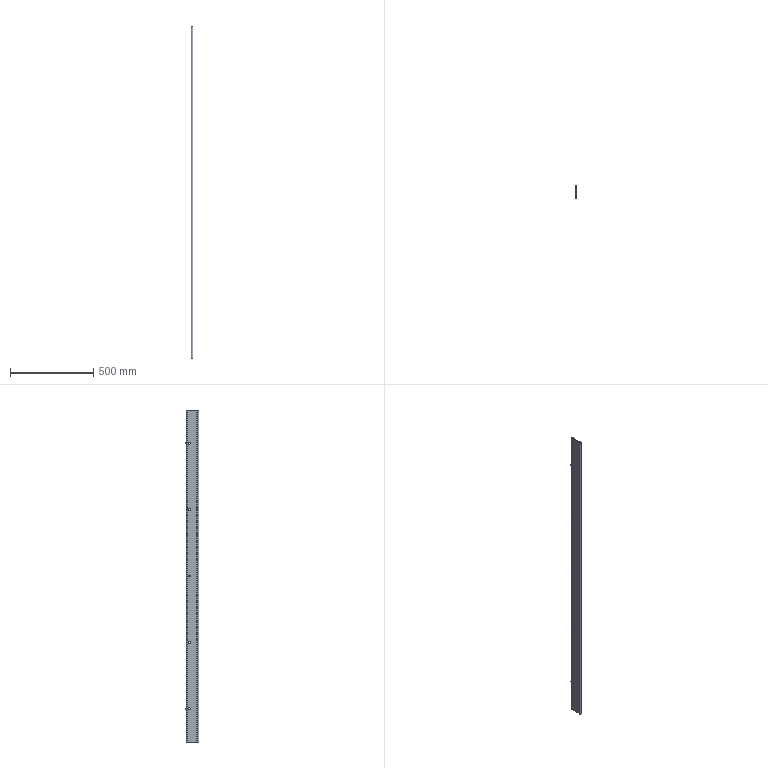Part | SolidWorks | features ICE 2, Extrusion 1 | 1 solid | 26 faces | box 12 x 81 x 2000 mm | volume 931360 mm3 | cylinder 20 | plane 6 | commonest cylinder face diameters 12 x13 6.5 x4 8 x3
STEP:
#1=CARTESIAN_POINT('',(0.,10.,1803.25));
#2=VERTEX_POINT('',#1);
#3=CARTESIAN_POINT('',(0.,10.,1796.75));
#4=VERTEX_POINT('',#3);
#5=CARTESIAN_POINT('',(0.,10.,1800.));
#6=DIRECTION('',(0.,1.,0.));
#7=DIRECTION('',(0.,0.,1.));
#8=AXIS2_PLACEMENT_3D('',#5,#6,#7);
#9=CIRCLE('',#8,3.25);
#10=EDGE_CURVE('',#2,#4,#9,.T.);
#11=ORIENTED_EDGE('',*,*,#10,.F.);
#12=CARTESIAN_POINT('',(0.,4.,1803.25));
#13=VERTEX_POINT('',#12);
#14=CARTESIAN_POINT('',(0.,10.,1803.25));
#15=DIRECTION('',(0.,-1.,0.));
#16=VECTOR('',#15,1000.);
#17=LINE('',#14,#16);
#18=EDGE_CURVE('',#2,#13,#17,.T.);
#19=ORIENTED_EDGE('',*,*,#18,.T.);
#20=CARTESIAN_POINT('',(0.,4.,1796.75));
#21=VERTEX_POINT('',#20);
#22=CARTESIAN_POINT('',(0.,4.,1803.25));
#23=CARTESIAN_POINT('',(0.2246,4.,1803.25));
#24=CARTESIAN_POINT('',(0.4531,3.98,1803.226));
#25=CARTESIAN_POINT('',(0.8876,3.906,1803.134));
#26=CARTESIAN_POINT('',(1.099,3.852,1803.066));
#27=CARTESIAN_POINT('',(1.693,3.648,1802.808));
#28=CARTESIAN_POINT('',(2.037,3.46,1802.564));
#29=CARTESIAN_POINT('',(2.599,3.06,1801.992));
#30=CARTESIAN_POINT('',(2.826,2.841,1801.656));
#31=CARTESIAN_POINT('',(3.068,2.57,1801.092));
#32=CARTESIAN_POINT('',(3.133,2.488,1800.892));
#33=CARTESIAN_POINT('',(3.225,2.368,1800.461));
#34=CARTESIAN_POINT('',(3.249,2.333,1800.237));
#35=CARTESIAN_POINT('',(3.251,2.331,1799.78));
#36=CARTESIAN_POINT('',(3.227,2.365,1799.557));
#37=CARTESIAN_POINT('',(3.138,2.482,1799.125));
#38=CARTESIAN_POINT('',(3.074,2.563,1798.924));
#39=CARTESIAN_POINT('',(2.912,2.745,1798.542));
#40=CARTESIAN_POINT('',(2.814,2.847,1798.362));
#41=CARTESIAN_POINT('',(2.591,3.051,1798.028));
#42=CARTESIAN_POINT('',(2.466,3.155,1797.873));
#43=CARTESIAN_POINT('',(2.183,3.357,1797.583));
#44=CARTESIAN_POINT('',(2.025,3.455,1797.45));
#45=CARTESIAN_POINT('',(1.685,3.633,1797.213));
#46=CARTESIAN_POINT('',(1.501,3.714,1797.109));
#47=CARTESIAN_POINT('',(1.102,3.851,1796.935));
#48=CARTESIAN_POINT('',(0.894,3.905,1796.867));
#49=CARTESIAN_POINT('',(0.4573,3.98,1796.775));
#50=CARTESIAN_POINT('',(0.2279,4.,1796.75));
#51=CARTESIAN_POINT('',(0.,4.,1796.75));
#52=B_SPLINE_CURVE_WITH_KNOTS('',3,(#22,#23,#24,#25,#26,#27,#28,#29,#30,#31,#32,#33,#34,#35,#36,#37,#38,#39,#40,#41,#42,#43,#44,#45,#46,#47,#48,#49,#50,#51),.UNSPECIFIED.,.F.,.F.,(4,2,2,2,2,2,2,2,2,2,2,2,2,2,4),(0.01079,0.01147,0.01214,0.01348,0.01483,0.0155,0.01617,0.01685,0.01752,0.01819,0.01886,0.01954,0.02021,0.02088,0.02155),.UNSPECIFIED.);
#53=EDGE_CURVE('',#13,#21,#52,.T.);
#54=ORIENTED_EDGE('',*,*,#53,.T.);
#55=CARTESIAN_POINT('',(0.,10.,1796.75));
#56=DIRECTION('',(0.,-1.,0.));
#57=VECTOR('',#56,1000.);
#58=LINE('',#55,#57);
#59=EDGE_CURVE('',#4,#21,#58,.T.);
#60=ORIENTED_EDGE('',*,*,#59,.F.);
#61=EDGE_LOOP('',(#11,#19,#54,#60));
#62=FACE_OUTER_BOUND('',#61,.T.);
#63=CARTESIAN_POINT('',(0.,10.,1800.));
#64=DIRECTION('',(0.,-1.,0.));
#65=DIRECTION('',(0.,0.,-1.));
#66=AXIS2_PLACEMENT_3D('',#63,#64,#65);
#67=CYLINDRICAL_SURFACE('',#66,3.25);
#68=ADVANCED_FACE('',(#62),#67,.T.);
#69=CARTESIAN_POINT('',(0.,10.,203.25));
#70=VERTEX_POINT('',#69);
#71=CARTESIAN_POINT('',(0.,10.,196.75));
#72=VERTEX_POINT('',#71);
#73=CARTESIAN_POINT('',(0.,10.,200.));
#74=DIRECTION('',(0.,1.,0.));
#75=DIRECTION('',(0.,0.,1.));
#76=AXIS2_PLACEMENT_3D('',#73,#74,#75);
#77=CIRCLE('',#76,3.25);
#78=EDGE_CURVE('',#70,#72,#77,.T.);
#79=ORIENTED_EDGE('',*,*,#78,.F.);
#80=CARTESIAN_POINT('',(0.,4.,203.25));
#81=VERTEX_POINT('',#80);
#82=CARTESIAN_POINT('',(0.,10.,203.25));
#83=DIRECTION('',(0.,-1.,0.));
#84=VECTOR('',#83,1000.);
#85=LINE('',#82,#84);
#86=EDGE_CURVE('',#70,#81,#85,.T.);
#87=ORIENTED_EDGE('',*,*,#86,.T.);
#88=CARTESIAN_POINT('',(0.,4.,196.75));
#89=VERTEX_POINT('',#88);
#90=CARTESIAN_POINT('',(0.,4.,203.25));
#91=CARTESIAN_POINT('',(0.2246,4.,203.25));
#92=CARTESIAN_POINT('',(0.4531,3.98,203.226));
#93=CARTESIAN_POINT('',(0.8876,3.906,203.134));
#94=CARTESIAN_POINT('',(1.099,3.852,203.066));
#95=CARTESIAN_POINT('',(1.693,3.648,202.808));
#96=CARTESIAN_POINT('',(2.037,3.46,202.564));
#97=CARTESIAN_POINT('',(2.599,3.06,201.992));
#98=CARTESIAN_POINT('',(2.826,2.841,201.656));
#99=CARTESIAN_POINT('',(3.068,2.57,201.092));
#100=CARTESIAN_POINT('',(3.133,2.488,200.892));
#101=CARTESIAN_POINT('',(3.225,2.368,200.461));
#102=CARTESIAN_POINT('',(3.249,2.333,200.237));
#103=CARTESIAN_POINT('',(3.251,2.331,199.78));
#104=CARTESIAN_POINT('',(3.227,2.365,199.557));
#105=CARTESIAN_POINT('',(3.138,2.482,199.125));
#106=CARTESIAN_POINT('',(3.074,2.563,198.924));
#107=CARTESIAN_POINT('',(2.912,2.745,198.542));
#108=CARTESIAN_POINT('',(2.814,2.847,198.362));
#109=CARTESIAN_POINT('',(2.591,3.051,198.028));
#110=CARTESIAN_POINT('',(2.466,3.155,197.873));
#111=CARTESIAN_POINT('',(2.183,3.357,197.583));
#112=CARTESIAN_POINT('',(2.025,3.455,197.45));
#113=CARTESIAN_POINT('',(1.685,3.633,197.213));
#114=CARTESIAN_POINT('',(1.501,3.714,197.109));
#115=CARTESIAN_POINT('',(1.102,3.851,196.935));
#116=CARTESIAN_POINT('',(0.894,3.905,196.867));
#117=CARTESIAN_POINT('',(0.4573,3.98,196.775));
#118=CARTESIAN_POINT('',(0.2279,4.,196.75));
#119=CARTESIAN_POINT('',(0.,4.,196.75));
#120=B_SPLINE_CURVE_WITH_KNOTS('',3,(#90,#91,#92,#93,#94,#95,#96,#97,#98,#99,#100,#101,#102,#103,#104,#105,#106,#107,#108,#109,#110,#111,#112,#113,#114,#115,#116,#117,#118,#119),.UNSPECIFIED.,.F.,.F.,(4,2,2,2,2,2,2,2,2,2,2,2,2,2,4),(0.01079,0.01147,0.01214,0.01348,0.01483,0.0155,0.01617,0.01685,0.01752,0.01819,0.01886,0.01954,0.02021,0.02088,0.02155),.UNSPECIFIED.);
#121=EDGE_CURVE('',#81,#89,#120,.T.);
#122=ORIENTED_EDGE('',*,*,#121,.T.);
#123=CARTESIAN_POINT('',(0.,10.,196.75));
#124=DIRECTION('',(0.,-1.,0.));
#125=VECTOR('',#124,1000.);
#126=LINE('',#123,#125);
#127=EDGE_CURVE('',#72,#89,#126,.T.);
#128=ORIENTED_EDGE('',*,*,#127,.F.);
#129=EDGE_LOOP('',(#79,#87,#122,#128));
#130=FACE_OUTER_BOUND('',#129,.T.);
#131=CARTESIAN_POINT('',(0.,10.,200.));
#132=DIRECTION('',(0.,-1.,0.));
#133=DIRECTION('',(0.,0.,-1.));
#134=AXIS2_PLACEMENT_3D('',#131,#132,#133);
#135=CYLINDRICAL_SURFACE('',#134,3.25);
#136=ADVANCED_FACE('',(#130),#135,.T.);
#137=CARTESIAN_POINT('',(-2.788,-20.971,600.));
#138=VERTEX_POINT('',#137);
#139=CARTESIAN_POINT('',(-2.788,-8.971,600.));
#140=VERTEX_POINT('',#139);
#141=CARTESIAN_POINT('',(-2.788,-14.971,600.));
#142=DIRECTION('',(1.,0.,0.));
#143=DIRECTION('',(0.,1.,0.));
#144=AXIS2_PLACEMENT_3D('',#141,#142,#143);
#145=CIRCLE('',#144,6.);
#146=EDGE_CURVE('',#138,#140,#145,.T.);
#147=ORIENTED_EDGE('',*,*,#146,.F.);
#148=CARTESIAN_POINT('',(2.678,-20.971,600.));
#149=VERTEX_POINT('',#148);
#150=CARTESIAN_POINT('',(-6.,-20.971,600.));
#151=DIRECTION('',(1.,0.,0.));
#152=VECTOR('',#151,1000.);
#153=LINE('',#150,#152);
#154=EDGE_CURVE('',#138,#149,#153,.T.);
#155=ORIENTED_EDGE('',*,*,#154,.T.);
#156=CARTESIAN_POINT('',(2.678,-8.971,600.));
#157=VERTEX_POINT('',#156);
#158=CARTESIAN_POINT('',(2.678,-14.971,600.));
#159=DIRECTION('',(1.,0.,0.));
#160=DIRECTION('',(0.,1.,0.));
#161=AXIS2_PLACEMENT_3D('',#158,#159,#160);
#162=CIRCLE('',#161,6.);
#163=EDGE_CURVE('',#149,#157,#162,.T.);
#164=ORIENTED_EDGE('',*,*,#163,.T.);
#165=CARTESIAN_POINT('',(-6.,-8.971,600.));
#166=DIRECTION('',(1.,0.,0.));
#167=VECTOR('',#166,1000.);
#168=LINE('',#165,#167);
#169=EDGE_CURVE('',#140,#157,#168,.T.);
#170=ORIENTED_EDGE('',*,*,#169,.F.);
#171=EDGE_LOOP('',(#147,#155,#164,#170));
#172=FACE_OUTER_BOUND('',#171,.T.);
#173=CARTESIAN_POINT('',(-6.,-14.971,600.));
#174=DIRECTION('',(1.,0.,0.));
#175=DIRECTION('',(0.,1.,0.));
#176=AXIS2_PLACEMENT_3D('',#173,#174,#175);
#177=CYLINDRICAL_SURFACE('',#176,6.);
#178=ADVANCED_FACE('',(#172),#177,.F.);
#179=CARTESIAN_POINT('',(-2.788,-20.971,1000.));
#180=VERTEX_POINT('',#179);
#181=CARTESIAN_POINT('',(-2.788,-8.971,1000.));
#182=VERTEX_POINT('',#181);
#183=CARTESIAN_POINT('',(-2.788,-14.971,1000.));
#184=DIRECTION('',(1.,0.,0.));
#185=DIRECTION('',(0.,1.,0.));
#186=AXIS2_PLACEMENT_3D('',#183,#184,#185);
#187=CIRCLE('',#186,6.);
#188=EDGE_CURVE('',#180,#182,#187,.T.);
#189=ORIENTED_EDGE('',*,*,#188,.F.);
#190=CARTESIAN_POINT('',(2.678,-20.971,1000.));
#191=VERTEX_POINT('',#190);
#192=CARTESIAN_POINT('',(-6.,-20.971,1000.));
#193=DIRECTION('',(1.,0.,0.));
#194=VECTOR('',#193,1000.);
#195=LINE('',#192,#194);
#196=EDGE_CURVE('',#180,#191,#195,.T.);
#197=ORIENTED_EDGE('',*,*,#196,.T.);
#198=CARTESIAN_POINT('',(2.678,-8.971,1000.));
#199=VERTEX_POINT('',#198);
#200=CARTESIAN_POINT('',(2.678,-14.971,1000.));
#201=DIRECTION('',(1.,0.,0.));
#202=DIRECTION('',(0.,1.,0.));
#203=AXIS2_PLACEMENT_3D('',#200,#201,#202);
#204=CIRCLE('',#203,6.);
#205=EDGE_CURVE('',#191,#199,#204,.T.);
#206=ORIENTED_EDGE('',*,*,#205,.T.);
#207=CARTESIAN_POINT('',(-6.,-8.971,1000.));
#208=DIRECTION('',(1.,0.,0.));
#209=VECTOR('',#208,1000.);
#210=LINE('',#207,#209);
#211=EDGE_CURVE('',#182,#199,#210,.T.);
#212=ORIENTED_EDGE('',*,*,#211,.F.);
#213=EDGE_LOOP('',(#189,#197,#206,#212));
#214=FACE_OUTER_BOUND('',#213,.T.);
#215=CARTESIAN_POINT('',(-6.,-14.971,1000.));
#216=DIRECTION('',(1.,0.,0.));
#217=DIRECTION('',(0.,1.,0.));
#218=AXIS2_PLACEMENT_3D('',#215,#216,#217);
#219=CYLINDRICAL_SURFACE('',#218,6.);
#220=ADVANCED_FACE('',(#214),#219,.F.);
#221=CARTESIAN_POINT('',(-2.788,-20.971,1400.));
#222=VERTEX_POINT('',#221);
#223=CARTESIAN_POINT('',(-2.788,-8.971,1400.));
#224=VERTEX_POINT('',#223);
#225=CARTESIAN_POINT('',(-2.788,-14.971,1400.));
#226=DIRECTION('',(1.,0.,0.));
#227=DIRECTION('',(0.,1.,0.));
#228=AXIS2_PLACEMENT_3D('',#225,#226,#227);
#229=CIRCLE('',#228,6.);
#230=EDGE_CURVE('',#222,#224,#229,.T.);
#231=ORIENTED_EDGE('',*,*,#230,.F.);
#232=CARTESIAN_POINT('',(2.678,-20.971,1400.));
#233=VERTEX_POINT('',#232);
#234=CARTESIAN_POINT('',(-6.,-20.971,1400.));
#235=DIRECTION('',(1.,0.,0.));
#236=VECTOR('',#235,1000.);
#237=LINE('',#234,#236);
#238=EDGE_CURVE('',#222,#233,#237,.T.);
#239=ORIENTED_EDGE('',*,*,#238,.T.);
#240=CARTESIAN_POINT('',(2.678,-8.971,1400.));
#241=VERTEX_POINT('',#240);
#242=CARTESIAN_POINT('',(2.678,-14.971,1400.));
#243=DIRECTION('',(1.,0.,0.));
#244=DIRECTION('',(0.,1.,0.));
#245=AXIS2_PLACEMENT_3D('',#242,#243,#244);
#246=CIRCLE('',#245,6.);
#247=EDGE_CURVE('',#233,#241,#246,.T.);
#248=ORIENTED_EDGE('',*,*,#247,.T.);
#249=CARTESIAN_POINT('',(-6.,-8.971,1400.));
#250=DIRECTION('',(1.,0.,0.));
#251=VECTOR('',#250,1000.);
#252=LINE('',#249,#251);
#253=EDGE_CURVE('',#224,#241,#252,.T.);
#254=ORIENTED_EDGE('',*,*,#253,.F.);
#255=EDGE_LOOP('',(#231,#239,#248,#254));
#256=FACE_OUTER_BOUND('',#255,.T.);
#257=CARTESIAN_POINT('',(-6.,-14.971,1400.));
#258=DIRECTION('',(1.,0.,0.));
#259=DIRECTION('',(0.,1.,0.));
#260=AXIS2_PLACEMENT_3D('',#257,#258,#259);
#261=CYLINDRICAL_SURFACE('',#260,6.);
#262=ADVANCED_FACE('',(#256),#261,.F.);
#263=CARTESIAN_POINT('',(-2.788,-20.971,1800.));
#264=VERTEX_POINT('',#263);
#265=CARTESIAN_POINT('',(-2.788,-8.971,1800.));
#266=VERTEX_POINT('',#265);
#267=CARTESIAN_POINT('',(-2.788,-14.971,1800.));
#268=DIRECTION('',(1.,0.,0.));
#269=DIRECTION('',(0.,1.,0.));
#270=AXIS2_PLACEMENT_3D('',#267,#268,#269);
#271=CIRCLE('',#270,6.);
#272=EDGE_CURVE('',#264,#266,#271,.T.);
#273=ORIENTED_EDGE('',*,*,#272,.F.);
#274=CARTESIAN_POINT('',(2.678,-20.971,1800.));
#275=VERTEX_POINT('',#274);
#276=CARTESIAN_POINT('',(-6.,-20.971,1800.));
#277=DIRECTION('',(1.,0.,0.));
#278=VECTOR('',#277,1000.);
#279=LINE('',#276,#278);
#280=EDGE_CURVE('',#264,#275,#279,.T.);
#281=ORIENTED_EDGE('',*,*,#280,.T.);
#282=CARTESIAN_POINT('',(2.678,-8.971,1800.));
#283=VERTEX_POINT('',#282);
#284=CARTESIAN_POINT('',(2.678,-14.971,1800.));
#285=DIRECTION('',(1.,0.,0.));
#286=DIRECTION('',(0.,1.,0.));
#287=AXIS2_PLACEMENT_3D('',#284,#285,#286);
#288=CIRCLE('',#287,6.);
#289=EDGE_CURVE('',#275,#283,#288,.T.);
#290=ORIENTED_EDGE('',*,*,#289,.T.);
#291=CARTESIAN_POINT('',(-6.,-8.971,1800.));
#292=DIRECTION('',(1.,0.,0.));
#293=VECTOR('',#292,1000.);
#294=LINE('',#291,#293);
#295=EDGE_CURVE('',#266,#283,#294,.T.);
#296=ORIENTED_EDGE('',*,*,#295,.F.);
#297=EDGE_LOOP('',(#273,#281,#290,#296));
#298=FACE_OUTER_BOUND('',#297,.T.);
#299=CARTESIAN_POINT('',(-6.,-14.971,1800.));
#300=DIRECTION('',(1.,0.,0.));
#301=DIRECTION('',(0.,1.,0.));
#302=AXIS2_PLACEMENT_3D('',#299,#300,#301);
#303=CYLINDRICAL_SURFACE('',#302,6.);
#304=ADVANCED_FACE('',(#298),#303,.F.);
#305=CARTESIAN_POINT('',(-2.788,-20.971,200.));
#306=VERTEX_POINT('',#305);
#307=CARTESIAN_POINT('',(-2.788,-8.971,200.));
#308=VERTEX_POINT('',#307);
#309=CARTESIAN_POINT('',(-2.788,-14.971,200.));
#310=DIRECTION('',(1.,0.,0.));
#311=DIRECTION('',(0.,1.,0.));
#312=AXIS2_PLACEMENT_3D('',#309,#310,#311);
#313=CIRCLE('',#312,6.);
#314=EDGE_CURVE('',#306,#308,#313,.T.);
#315=ORIENTED_EDGE('',*,*,#314,.F.);
#316=CARTESIAN_POINT('',(2.678,-20.971,200.));
#317=VERTEX_POINT('',#316);
#318=CARTESIAN_POINT('',(-6.,-20.971,200.));
#319=DIRECTION('',(1.,0.,0.));
#320=VECTOR('',#319,1000.);
#321=LINE('',#318,#320);
#322=EDGE_CURVE('',#306,#317,#321,.T.);
#323=ORIENTED_EDGE('',*,*,#322,.T.);
#324=CARTESIAN_POINT('',(2.678,-8.971,200.));
#325=VERTEX_POINT('',#324);
#326=CARTESIAN_POINT('',(2.678,-14.971,200.));
#327=DIRECTION('',(1.,0.,0.));
#328=DIRECTION('',(0.,1.,0.));
#329=AXIS2_PLACEMENT_3D('',#326,#327,#328);
#330=CIRCLE('',#329,6.);
#331=EDGE_CURVE('',#317,#325,#330,.T.);
#332=ORIENTED_EDGE('',*,*,#331,.T.);
#333=CARTESIAN_POINT('',(-6.,-8.971,200.));
#334=DIRECTION('',(1.,0.,0.));
#335=VECTOR('',#334,1000.);
#336=LINE('',#333,#335);
#337=EDGE_CURVE('',#308,#325,#336,.T.);
#338=ORIENTED_EDGE('',*,*,#337,.F.);
#339=EDGE_LOOP('',(#315,#323,#332,#338));
#340=FACE_OUTER_BOUND('',#339,.T.);
#341=CARTESIAN_POINT('',(-6.,-14.971,200.));
#342=DIRECTION('',(1.,0.,0.));
#343=DIRECTION('',(0.,1.,0.));
#344=AXIS2_PLACEMENT_3D('',#341,#342,#343);
#345=CYLINDRICAL_SURFACE('',#344,6.);
#346=ADVANCED_FACE('',(#340),#345,.F.);
#347=CARTESIAN_POINT('',(6.,-65.,2000.));
#348=VERTEX_POINT('',#347);
#349=CARTESIAN_POINT('',(2.678,-59.631,2000.));
#350=VERTEX_POINT('',#349);
#351=CARTESIAN_POINT('',(0.,-65.,2000.));
#352=DIRECTION('',(0.,0.,1.));
#353=DIRECTION('',(1.,0.,0.));
#354=AXIS2_PLACEMENT_3D('',#351,#352,#353);
#355=CIRCLE('',#354,6.);
#356=EDGE_CURVE('',#348,#350,#355,.T.);
#357=ORIENTED_EDGE('',*,*,#356,.F.);
#358=CARTESIAN_POINT('',(6.,-65.,0.));
#359=VERTEX_POINT('',#358);
#360=CARTESIAN_POINT('',(6.,-65.,2000.));
#361=DIRECTION('',(0.,0.,-1.));
#362=VECTOR('',#361,1000.);
#363=LINE('',#360,#362);
#364=EDGE_CURVE('',#348,#359,#363,.T.);
#365=ORIENTED_EDGE('',*,*,#364,.T.);
#366=CARTESIAN_POINT('',(2.678,-59.631,0.));
#367=VERTEX_POINT('',#366);
#368=CARTESIAN_POINT('',(0.,-65.,0.));
#369=DIRECTION('',(0.,0.,1.));
#370=DIRECTION('',(1.,0.,0.));
#371=AXIS2_PLACEMENT_3D('',#368,#369,#370);
#372=CIRCLE('',#371,6.);
#373=EDGE_CURVE('',#359,#367,#372,.T.);
#374=ORIENTED_EDGE('',*,*,#373,.T.);
#375=CARTESIAN_POINT('',(2.678,-59.631,2000.));
#376=DIRECTION('',(0.,0.,-1.));
#377=VECTOR('',#376,1000.);
#378=LINE('',#375,#377);
#379=EDGE_CURVE('',#350,#367,#378,.T.);
#380=ORIENTED_EDGE('',*,*,#379,.F.);
#381=EDGE_LOOP('',(#357,#365,#374,#380));
#382=FACE_OUTER_BOUND('',#381,.T.);
#383=CARTESIAN_POINT('',(0.,-65.,2000.));
#384=DIRECTION('',(0.,0.,-1.));
#385=DIRECTION('',(-1.,0.,0.));
#386=AXIS2_PLACEMENT_3D('',#383,#384,#385);
#387=CYLINDRICAL_SURFACE('',#386,6.);
#388=ADVANCED_FACE('',(#382),#387,.T.);
#389=ORIENTED_EDGE('',*,*,#364,.F.);
#390=CARTESIAN_POINT('',(-6.,-65.,2000.));
#391=VERTEX_POINT('',#390);
#392=CARTESIAN_POINT('',(0.,-65.,2000.));
#393=DIRECTION('',(0.,0.,1.));
#394=DIRECTION('',(1.,0.,0.));
#395=AXIS2_PLACEMENT_3D('',#392,#393,#394);
#396=CIRCLE('',#395,6.);
#397=EDGE_CURVE('',#391,#348,#396,.T.);
#398=ORIENTED_EDGE('',*,*,#397,.F.);
#399=CARTESIAN_POINT('',(-6.,-65.,0.));
#400=VERTEX_POINT('',#399);
#401=CARTESIAN_POINT('',(-6.,-65.,2000.));
#402=DIRECTION('',(0.,0.,-1.));
#403=VECTOR('',#402,1000.);
#404=LINE('',#401,#403);
#405=EDGE_CURVE('',#391,#400,#404,.T.);
#406=ORIENTED_EDGE('',*,*,#405,.T.);
#407=CARTESIAN_POINT('',(0.,-65.,0.));
#408=DIRECTION('',(0.,0.,1.));
#409=DIRECTION('',(1.,0.,0.));
#410=AXIS2_PLACEMENT_3D('',#407,#408,#409);
#411=CIRCLE('',#410,6.);
#412=EDGE_CURVE('',#400,#359,#411,.T.);
#413=ORIENTED_EDGE('',*,*,#412,.T.);
#414=EDGE_LOOP('',(#389,#398,#406,#413));
#415=FACE_OUTER_BOUND('',#414,.T.);
#416=CARTESIAN_POINT('',(0.,-65.,2000.));
#417=DIRECTION('',(0.,0.,-1.));
#418=DIRECTION('',(-1.,0.,0.));
#419=AXIS2_PLACEMENT_3D('',#416,#417,#418);
#420=CYLINDRICAL_SURFACE('',#419,6.);
#421=ADVANCED_FACE('',(#415),#420,.T.);
#422=CARTESIAN_POINT('',(0.,4.,196.75));
#423=CARTESIAN_POINT('',(-0.2287,4.,196.75));
#424=CARTESIAN_POINT('',(-0.4517,3.981,196.774));
#425=CARTESIAN_POINT('',(-0.8873,3.907,196.866));
#426=CARTESIAN_POINT('',(-1.1,3.851,196.934));
#427=CARTESIAN_POINT('',(-1.495,3.716,197.106));
#428=CARTESIAN_POINT('',(-1.681,3.635,197.211));
#429=CARTESIAN_POINT('',(-2.023,3.456,197.448));
#430=CARTESIAN_POINT('',(-2.178,3.359,197.579));
#431=CARTESIAN_POINT('',(-2.46,3.159,197.867));
#432=CARTESIAN_POINT('',(-2.589,3.053,198.025));
#433=CARTESIAN_POINT('',(-2.812,2.848,198.359));
#434=CARTESIAN_POINT('',(-2.909,2.748,198.536));
#435=CARTESIAN_POINT('',(-3.07,2.567,198.915));
#436=CARTESIAN_POINT('',(-3.136,2.484,199.12));
#437=CARTESIAN_POINT('',(-3.226,2.366,199.548));
#438=CARTESIAN_POINT('',(-3.25,2.332,199.776));
#439=CARTESIAN_POINT('',(-3.25,2.332,200.227));
#440=CARTESIAN_POINT('',(-3.225,2.367,200.454));
#441=CARTESIAN_POINT('',(-3.136,2.484,200.882));
#442=CARTESIAN_POINT('',(-3.071,2.566,201.084));
#443=CARTESIAN_POINT('',(-2.908,2.75,201.467));
#444=CARTESIAN_POINT('',(-2.811,2.85,201.643));
#445=CARTESIAN_POINT('',(-2.588,3.054,201.977));
#446=CARTESIAN_POINT('',(-2.46,3.159,202.134));
#447=CARTESIAN_POINT('',(-2.176,3.361,202.423));
#448=CARTESIAN_POINT('',(-2.021,3.457,202.554));
#449=CARTESIAN_POINT('',(-1.682,3.634,202.789));
#450=CARTESIAN_POINT('',(-1.494,3.716,202.894));
#451=CARTESIAN_POINT('',(-1.099,3.852,203.066));
#452=CARTESIAN_POINT('',(-0.8903,3.906,203.134));
#453=CARTESIAN_POINT('',(-0.4494,3.981,203.227));
#454=CARTESIAN_POINT('',(-0.2254,4.,203.25));
#455=CARTESIAN_POINT('',(0.,4.,203.25));
#456=B_SPLINE_CURVE_WITH_KNOTS('',3,(#422,#423,#424,#425,#426,#427,#428,#429,#430,#431,#432,#433,#434,#435,#436,#437,#438,#439,#440,#441,#442,#443,#444,#445,#446,#447,#448,#449,#450,#451,#452,#453,#454,#455),.UNSPECIFIED.,.F.,.F.,(4,2,2,2,2,2,2,2,2,2,2,2,2,2,2,2,4),(0.,0.0006746,0.001349,0.002024,0.002699,0.003373,0.004048,0.004723,0.005397,0.006072,0.006746,0.007421,0.008096,0.00877,0.009445,0.01012,0.01079),.UNSPECIFIED.);
#457=EDGE_CURVE('',#89,#81,#456,.T.);
#458=ORIENTED_EDGE('',*,*,#457,.F.);
#459=ORIENTED_EDGE('',*,*,#121,.F.);
#460=EDGE_LOOP('',(#458,#459));
#461=FACE_BOUND('',#460,.T.);
#462=CARTESIAN_POINT('',(0.,4.,1796.75));
#463=CARTESIAN_POINT('',(-0.2287,4.,1796.75));
#464=CARTESIAN_POINT('',(-0.4517,3.981,1796.774));
#465=CARTESIAN_POINT('',(-0.8873,3.907,1796.866));
#466=CARTESIAN_POINT('',(-1.1,3.851,1796.934));
#467=CARTESIAN_POINT('',(-1.495,3.716,1797.106));
#468=CARTESIAN_POINT('',(-1.681,3.635,1797.211));
#469=CARTESIAN_POINT('',(-2.023,3.456,1797.448));
#470=CARTESIAN_POINT('',(-2.178,3.359,1797.579));
#471=CARTESIAN_POINT('',(-2.46,3.159,1797.867));
#472=CARTESIAN_POINT('',(-2.589,3.053,1798.025));
#473=CARTESIAN_POINT('',(-2.812,2.848,1798.359));
#474=CARTESIAN_POINT('',(-2.909,2.748,1798.536));
#475=CARTESIAN_POINT('',(-3.07,2.567,1798.915));
#476=CARTESIAN_POINT('',(-3.136,2.484,1799.12));
#477=CARTESIAN_POINT('',(-3.226,2.366,1799.548));
#478=CARTESIAN_POINT('',(-3.25,2.332,1799.776));
#479=CARTESIAN_POINT('',(-3.25,2.332,1800.227));
#480=CARTESIAN_POINT('',(-3.225,2.367,1800.454));
#481=CARTESIAN_POINT('',(-3.136,2.484,1800.882));
#482=CARTESIAN_POINT('',(-3.071,2.566,1801.084));
#483=CARTESIAN_POINT('',(-2.908,2.75,1801.467));
#484=CARTESIAN_POINT('',(-2.811,2.85,1801.643));
#485=CARTESIAN_POINT('',(-2.588,3.054,1801.977));
#486=CARTESIAN_POINT('',(-2.46,3.159,1802.134));
#487=CARTESIAN_POINT('',(-2.176,3.361,1802.423));
#488=CARTESIAN_POINT('',(-2.021,3.457,1802.554));
#489=CARTESIAN_POINT('',(-1.682,3.634,1802.789));
#490=CARTESIAN_POINT('',(-1.494,3.716,1802.894));
#491=CARTESIAN_POINT('',(-1.099,3.852,1803.066));
#492=CARTESIAN_POINT('',(-0.8903,3.906,1803.134));
#493=CARTESIAN_POINT('',(-0.4494,3.981,1803.227));
#494=CARTESIAN_POINT('',(-0.2254,4.,1803.25));
#495=CARTESIAN_POINT('',(0.,4.,1803.25));
#496=B_SPLINE_CURVE_WITH_KNOTS('',3,(#462,#463,#464,#465,#466,#467,#468,#469,#470,#471,#472,#473,#474,#475,#476,#477,#478,#479,#480,#481,#482,#483,#484,#485,#486,#487,#488,#489,#490,#491,#492,#493,#494,#495),.UNSPECIFIED.,.F.,.F.,(4,2,2,2,2,2,2,2,2,2,2,2,2,2,2,2,4),(0.,0.0006746,0.001349,0.002024,0.002699,0.003373,0.004048,0.004723,0.005397,0.006072,0.006746,0.007421,0.008096,0.00877,0.009445,0.01012,0.01079),.UNSPECIFIED.);
#497=EDGE_CURVE('',#21,#13,#496,.T.);
#498=ORIENTED_EDGE('',*,*,#497,.F.);
#499=ORIENTED_EDGE('',*,*,#53,.F.);
#500=EDGE_LOOP('',(#498,#499));
#501=FACE_BOUND('',#500,.T.);
#502=CARTESIAN_POINT('',(4.,0.,2000.));
#503=VERTEX_POINT('',#502);
#504=CARTESIAN_POINT('',(-4.,0.,2000.));
#505=VERTEX_POINT('',#504);
#506=CARTESIAN_POINT('',(0.,0.,2000.));
#507=DIRECTION('',(0.,0.,1.));
#508=DIRECTION('',(1.,0.,0.));
#509=AXIS2_PLACEMENT_3D('',#506,#507,#508);
#510=CIRCLE('',#509,4.);
#511=EDGE_CURVE('',#503,#505,#510,.T.);
#512=ORIENTED_EDGE('',*,*,#511,.F.);
#513=CARTESIAN_POINT('',(4.,0.,0.));
#514=VERTEX_POINT('',#513);
#515=CARTESIAN_POINT('',(4.,0.,2000.));
#516=DIRECTION('',(0.,0.,-1.));
#517=VECTOR('',#516,1000.);
#518=LINE('',#515,#517);
#519=EDGE_CURVE('',#503,#514,#518,.T.);
#520=ORIENTED_EDGE('',*,*,#519,.T.);
#521=CARTESIAN_POINT('',(-4.,0.,0.));
#522=VERTEX_POINT('',#521);
#523=CARTESIAN_POINT('',(0.,0.,0.));
#524=DIRECTION('',(0.,0.,1.));
#525=DIRECTION('',(1.,0.,0.));
#526=AXIS2_PLACEMENT_3D('',#523,#524,#525);
#527=CIRCLE('',#526,4.);
#528=EDGE_CURVE('',#514,#522,#527,.T.);
#529=ORIENTED_EDGE('',*,*,#528,.T.);
#530=CARTESIAN_POINT('',(-4.,0.,2000.));
#531=DIRECTION('',(0.,0.,-1.));
#532=VECTOR('',#531,1000.);
#533=LINE('',#530,#532);
#534=EDGE_CURVE('',#505,#522,#533,.T.);
#535=ORIENTED_EDGE('',*,*,#534,.F.);
#536=EDGE_LOOP('',(#512,#520,#529,#535));
#537=FACE_OUTER_BOUND('',#536,.T.);
#538=CARTESIAN_POINT('',(0.,0.,2000.));
#539=DIRECTION('',(0.,0.,-1.));
#540=DIRECTION('',(-1.,0.,0.));
#541=AXIS2_PLACEMENT_3D('',#538,#539,#540);
#542=CYLINDRICAL_SURFACE('',#541,4.);
#543=ADVANCED_FACE('',(#461,#501,#537),#542,.T.);
#544=CARTESIAN_POINT('',(-2.788,-2.868,2000.));
#545=VERTEX_POINT('',#544);
#546=CARTESIAN_POINT('',(0.,0.,2000.));
#547=DIRECTION('',(0.,0.,1.));
#548=DIRECTION('',(1.,0.,0.));
#549=AXIS2_PLACEMENT_3D('',#546,#547,#548);
#550=CIRCLE('',#549,4.);
#551=EDGE_CURVE('',#505,#545,#550,.T.);
#552=ORIENTED_EDGE('',*,*,#551,.F.);
#553=ORIENTED_EDGE('',*,*,#534,.T.);
#554=CARTESIAN_POINT('',(-2.788,-2.868,0.));
#555=VERTEX_POINT('',#554);
#556=CARTESIAN_POINT('',(0.,0.,0.));
#557=DIRECTION('',(0.,0.,1.));
#558=DIRECTION('',(1.,0.,0.));
#559=AXIS2_PLACEMENT_3D('',#556,#557,#558);
#560=CIRCLE('',#559,4.);
#561=EDGE_CURVE('',#522,#555,#560,.T.);
#562=ORIENTED_EDGE('',*,*,#561,.T.);
#563=CARTESIAN_POINT('',(-2.788,-2.868,2000.));
#564=DIRECTION('',(0.,0.,-1.));
#565=VECTOR('',#564,1000.);
#566=LINE('',#563,#565);
#567=EDGE_CURVE('',#545,#555,#566,.T.);
#568=ORIENTED_EDGE('',*,*,#567,.F.);
#569=EDGE_LOOP('',(#552,#553,#562,#568));
#570=FACE_OUTER_BOUND('',#569,.T.);
#571=CARTESIAN_POINT('',(0.,0.,2000.));
#572=DIRECTION('',(0.,0.,-1.));
#573=DIRECTION('',(-1.,0.,0.));
#574=AXIS2_PLACEMENT_3D('',#571,#572,#573);
#575=CYLINDRICAL_SURFACE('',#574,4.);
#576=ADVANCED_FACE('',(#570),#575,.T.);
#577=ORIENTED_EDGE('',*,*,#519,.F.);
#578=CARTESIAN_POINT('',(2.678,-2.971,2000.));
#579=VERTEX_POINT('',#578);
#580=CARTESIAN_POINT('',(0.,0.,2000.));
#581=DIRECTION('',(0.,0.,1.));
#582=DIRECTION('',(1.,0.,0.));
#583=AXIS2_PLACEMENT_3D('',#580,#581,#582);
#584=CIRCLE('',#583,4.);
#585=EDGE_CURVE('',#579,#503,#584,.T.);
#586=ORIENTED_EDGE('',*,*,#585,.F.);
#587=CARTESIAN_POINT('',(2.678,-2.971,0.));
#588=VERTEX_POINT('',#587);
#589=CARTESIAN_POINT('',(2.678,-2.971,2000.));
#590=DIRECTION('',(0.,0.,-1.));
#591=VECTOR('',#590,1000.);
#592=LINE('',#589,#591);
#593=EDGE_CURVE('',#579,#588,#592,.T.);
#594=ORIENTED_EDGE('',*,*,#593,.T.);
#595=CARTESIAN_POINT('',(0.,0.,0.));
#596=DIRECTION('',(0.,0.,1.));
#597=DIRECTION('',(1.,0.,0.));
#598=AXIS2_PLACEMENT_3D('',#595,#596,#597);
#599=CIRCLE('',#598,4.);
#600=EDGE_CURVE('',#588,#514,#599,.T.);
#601=ORIENTED_EDGE('',*,*,#600,.T.);
#602=EDGE_LOOP('',(#577,#586,#594,#601));
#603=FACE_OUTER_BOUND('',#602,.T.);
#604=CARTESIAN_POINT('',(0.,0.,2000.));
#605=DIRECTION('',(0.,0.,-1.));
#606=DIRECTION('',(-1.,0.,0.));
#607=AXIS2_PLACEMENT_3D('',#604,#605,#606);
#608=CYLINDRICAL_SURFACE('',#607,4.);
#609=ADVANCED_FACE('',(#603),#608,.T.);
#610=ORIENTED_EDGE('',*,*,#405,.F.);
#611=CARTESIAN_POINT('',(-2.788,-59.687,2000.));
#612=VERTEX_POINT('',#611);
#613=CARTESIAN_POINT('',(0.,-65.,2000.));
#614=DIRECTION('',(0.,0.,1.));
#615=DIRECTION('',(1.,0.,0.));
#616=AXIS2_PLACEMENT_3D('',#613,#614,#615);
#617=CIRCLE('',#616,6.);
#618=EDGE_CURVE('',#612,#391,#617,.T.);
#619=ORIENTED_EDGE('',*,*,#618,.F.);
#620=CARTESIAN_POINT('',(-2.788,-59.687,0.));
#621=VERTEX_POINT('',#620);
#622=CARTESIAN_POINT('',(-2.788,-59.687,2000.));
#623=DIRECTION('',(0.,0.,-1.));
#624=VECTOR('',#623,1000.);
#625=LINE('',#622,#624);
#626=EDGE_CURVE('',#612,#621,#625,.T.);
#627=ORIENTED_EDGE('',*,*,#626,.T.);
#628=CARTESIAN_POINT('',(0.,-65.,0.));
#629=DIRECTION('',(0.,0.,1.));
#630=DIRECTION('',(1.,0.,0.));
#631=AXIS2_PLACEMENT_3D('',#628,#629,#630);
#632=CIRCLE('',#631,6.);
#633=EDGE_CURVE('',#621,#400,#632,.T.);
#634=ORIENTED_EDGE('',*,*,#633,.T.);
#635=EDGE_LOOP('',(#610,#619,#627,#634));
#636=FACE_OUTER_BOUND('',#635,.T.);
#637=CARTESIAN_POINT('',(0.,-65.,2000.));
#638=DIRECTION('',(0.,0.,-1.));
#639=DIRECTION('',(-1.,0.,0.));
#640=AXIS2_PLACEMENT_3D('',#637,#638,#639);
#641=CYLINDRICAL_SURFACE('',#640,6.);
#642=ADVANCED_FACE('',(#636),#641,.T.);
#643=CARTESIAN_POINT('',(2.678,-14.971,600.));
#644=DIRECTION('',(1.,0.,0.));
#645=DIRECTION('',(0.,1.,0.));
#646=AXIS2_PLACEMENT_3D('',#643,#644,#645);
#647=CIRCLE('',#646,6.);
#648=EDGE_CURVE('',#157,#149,#647,.T.);
#649=ORIENTED_EDGE('',*,*,#648,.F.);
#650=ORIENTED_EDGE('',*,*,#163,.F.);
#651=EDGE_LOOP('',(#649,#650));
#652=FACE_BOUND('',#651,.T.);
#653=CARTESIAN_POINT('',(2.678,-14.971,1000.));
#654=DIRECTION('',(1.,0.,0.));
#655=DIRECTION('',(0.,1.,0.));
#656=AXIS2_PLACEMENT_3D('',#653,#654,#655);
#657=CIRCLE('',#656,6.);
#658=EDGE_CURVE('',#199,#191,#657,.T.);
#659=ORIENTED_EDGE('',*,*,#658,.F.);
#660=ORIENTED_EDGE('',*,*,#205,.F.);
#661=EDGE_LOOP('',(#659,#660));
#662=FACE_BOUND('',#661,.T.);
#663=CARTESIAN_POINT('',(2.678,-14.971,1400.));
#664=DIRECTION('',(1.,0.,0.));
#665=DIRECTION('',(0.,1.,0.));
#666=AXIS2_PLACEMENT_3D('',#663,#664,#665);
#667=CIRCLE('',#666,6.);
#668=EDGE_CURVE('',#241,#233,#667,.T.);
#669=ORIENTED_EDGE('',*,*,#668,.F.);
#670=ORIENTED_EDGE('',*,*,#247,.F.);
#671=EDGE_LOOP('',(#669,#670));
#672=FACE_BOUND('',#671,.T.);
#673=CARTESIAN_POINT('',(2.678,-14.971,1800.));
#674=DIRECTION('',(1.,0.,0.));
#675=DIRECTION('',(0.,1.,0.));
#676=AXIS2_PLACEMENT_3D('',#673,#674,#675);
#677=CIRCLE('',#676,6.);
#678=EDGE_CURVE('',#283,#275,#677,.T.);
#679=ORIENTED_EDGE('',*,*,#678,.F.);
#680=ORIENTED_EDGE('',*,*,#289,.F.);
#681=EDGE_LOOP('',(#679,#680));
#682=FACE_BOUND('',#681,.T.);
#683=CARTESIAN_POINT('',(2.678,-14.971,200.));
#684=DIRECTION('',(1.,0.,0.));
#685=DIRECTION('',(0.,1.,0.));
#686=AXIS2_PLACEMENT_3D('',#683,#684,#685);
#687=CIRCLE('',#686,6.);
#688=EDGE_CURVE('',#325,#317,#687,.T.);
#689=ORIENTED_EDGE('',*,*,#688,.F.);
#690=ORIENTED_EDGE('',*,*,#331,.F.);
#691=EDGE_LOOP('',(#689,#690));
#692=FACE_BOUND('',#691,.T.);
#693=CARTESIAN_POINT('',(2.678,-2.971,0.));
#694=DIRECTION('',(0.,1.,0.));
#695=VECTOR('',#694,1000.);
#696=LINE('',#693,#695);
#697=EDGE_CURVE('',#367,#588,#696,.T.);
#698=ORIENTED_EDGE('',*,*,#697,.T.);
#699=ORIENTED_EDGE('',*,*,#593,.F.);
#700=CARTESIAN_POINT('',(2.678,-2.971,2000.));
#701=DIRECTION('',(0.,1.,0.));
#702=VECTOR('',#701,1000.);
#703=LINE('',#700,#702);
#704=EDGE_CURVE('',#350,#579,#703,.T.);
#705=ORIENTED_EDGE('',*,*,#704,.F.);
#706=ORIENTED_EDGE('',*,*,#379,.T.);
#707=EDGE_LOOP('',(#698,#699,#705,#706));
#708=FACE_OUTER_BOUND('',#707,.T.);
#709=CARTESIAN_POINT('',(2.678,-2.971,2000.));
#710=DIRECTION('',(-1.,0.,0.));
#711=DIRECTION('',(0.,-1.,0.));
#712=AXIS2_PLACEMENT_3D('',#709,#710,#711);
#713=PLANE('',#712);
#714=ADVANCED_FACE('',(#652,#662,#672,#682,#692,#708),#713,.F.);
#715=CARTESIAN_POINT('',(-2.788,-14.971,600.));
#716=DIRECTION('',(1.,0.,0.));
#717=DIRECTION('',(0.,1.,0.));
#718=AXIS2_PLACEMENT_3D('',#715,#716,#717);
#719=CIRCLE('',#718,6.);
#720=EDGE_CURVE('',#140,#138,#719,.T.);
#721=ORIENTED_EDGE('',*,*,#720,.T.);
#722=ORIENTED_EDGE('',*,*,#146,.T.);
#723=EDGE_LOOP('',(#721,#722));
#724=FACE_BOUND('',#723,.T.);
#725=CARTESIAN_POINT('',(-2.788,-14.971,1000.));
#726=DIRECTION('',(1.,0.,0.));
#727=DIRECTION('',(0.,1.,0.));
#728=AXIS2_PLACEMENT_3D('',#725,#726,#727);
#729=CIRCLE('',#728,6.);
#730=EDGE_CURVE('',#182,#180,#729,.T.);
#731=ORIENTED_EDGE('',*,*,#730,.T.);
#732=ORIENTED_EDGE('',*,*,#188,.T.);
#733=EDGE_LOOP('',(#731,#732));
#734=FACE_BOUND('',#733,.T.);
#735=CARTESIAN_POINT('',(-2.788,-14.971,1400.));
#736=DIRECTION('',(1.,0.,0.));
#737=DIRECTION('',(0.,1.,0.));
#738=AXIS2_PLACEMENT_3D('',#735,#736,#737);
#739=CIRCLE('',#738,6.);
#740=EDGE_CURVE('',#224,#222,#739,.T.);
#741=ORIENTED_EDGE('',*,*,#740,.T.);
#742=ORIENTED_EDGE('',*,*,#230,.T.);
#743=EDGE_LOOP('',(#741,#742));
#744=FACE_BOUND('',#743,.T.);
#745=CARTESIAN_POINT('',(-2.788,-14.971,1800.));
#746=DIRECTION('',(1.,0.,0.));
#747=DIRECTION('',(0.,1.,0.));
#748=AXIS2_PLACEMENT_3D('',#745,#746,#747);
#749=CIRCLE('',#748,6.);
#750=EDGE_CURVE('',#266,#264,#749,.T.);
#751=ORIENTED_EDGE('',*,*,#750,.T.);
#752=ORIENTED_EDGE('',*,*,#272,.T.);
#753=EDGE_LOOP('',(#751,#752));
#754=FACE_BOUND('',#753,.T.);
#755=CARTESIAN_POINT('',(-2.788,-14.971,200.));
#756=DIRECTION('',(1.,0.,0.));
#757=DIRECTION('',(0.,1.,0.));
#758=AXIS2_PLACEMENT_3D('',#755,#756,#757);
#759=CIRCLE('',#758,6.);
#760=EDGE_CURVE('',#308,#306,#759,.T.);
#761=ORIENTED_EDGE('',*,*,#760,.T.);
#762=ORIENTED_EDGE('',*,*,#314,.T.);
#763=EDGE_LOOP('',(#761,#762));
#764=FACE_BOUND('',#763,.T.);
#765=CARTESIAN_POINT('',(-2.788,-2.868,0.));
#766=DIRECTION('',(0.,-1.,0.));
#767=VECTOR('',#766,1000.);
#768=LINE('',#765,#767);
#769=EDGE_CURVE('',#555,#621,#768,.T.);
#770=ORIENTED_EDGE('',*,*,#769,.T.);
#771=ORIENTED_EDGE('',*,*,#626,.F.);
#772=CARTESIAN_POINT('',(-2.788,-2.868,2000.));
#773=DIRECTION('',(0.,-1.,0.));
#774=VECTOR('',#773,1000.);
#775=LINE('',#772,#774);
#776=EDGE_CURVE('',#545,#612,#775,.T.);
#777=ORIENTED_EDGE('',*,*,#776,.F.);
#778=ORIENTED_EDGE('',*,*,#567,.T.);
#779=EDGE_LOOP('',(#770,#771,#777,#778));
#780=FACE_OUTER_BOUND('',#779,.T.);
#781=CARTESIAN_POINT('',(-2.788,-2.868,2000.));
#782=DIRECTION('',(1.,0.,0.));
#783=DIRECTION('',(0.,1.,0.));
#784=AXIS2_PLACEMENT_3D('',#781,#782,#783);
#785=PLANE('',#784);
#786=ADVANCED_FACE('',(#724,#734,#744,#754,#764,#780),#785,.F.);
#787=ORIENTED_EDGE('',*,*,#618,.T.);
#788=ORIENTED_EDGE('',*,*,#397,.T.);
#789=ORIENTED_EDGE('',*,*,#356,.T.);
#790=ORIENTED_EDGE('',*,*,#704,.T.);
#791=ORIENTED_EDGE('',*,*,#585,.T.);
#792=ORIENTED_EDGE('',*,*,#511,.T.);
#793=ORIENTED_EDGE('',*,*,#551,.T.);
#794=ORIENTED_EDGE('',*,*,#776,.T.);
#795=EDGE_LOOP('',(#787,#788,#789,#790,#791,#792,#793,#794));
#796=FACE_OUTER_BOUND('',#795,.T.);
#797=CARTESIAN_POINT('',(0.,-65.,2000.));
#798=DIRECTION('',(0.,0.,1.));
#799=DIRECTION('',(1.,0.,0.));
#800=AXIS2_PLACEMENT_3D('',#797,#798,#799);
#801=PLANE('',#800);
#802=ADVANCED_FACE('',(#796),#801,.T.);
#803=ORIENTED_EDGE('',*,*,#633,.F.);
#804=ORIENTED_EDGE('',*,*,#769,.F.);
#805=ORIENTED_EDGE('',*,*,#561,.F.);
#806=ORIENTED_EDGE('',*,*,#528,.F.);
#807=ORIENTED_EDGE('',*,*,#600,.F.);
#808=ORIENTED_EDGE('',*,*,#697,.F.);
#809=ORIENTED_EDGE('',*,*,#373,.F.);
#810=ORIENTED_EDGE('',*,*,#412,.F.);
#811=EDGE_LOOP('',(#803,#804,#805,#806,#807,#808,#809,#810));
#812=FACE_OUTER_BOUND('',#811,.T.);
#813=CARTESIAN_POINT('',(0.,-65.,0.));
#814=DIRECTION('',(0.,0.,1.));
#815=DIRECTION('',(1.,0.,0.));
#816=AXIS2_PLACEMENT_3D('',#813,#814,#815);
#817=PLANE('',#816);
#818=ADVANCED_FACE('',(#812),#817,.F.);
#819=ORIENTED_EDGE('',*,*,#322,.F.);
#820=ORIENTED_EDGE('',*,*,#760,.F.);
#821=ORIENTED_EDGE('',*,*,#337,.T.);
#822=ORIENTED_EDGE('',*,*,#688,.T.);
#823=EDGE_LOOP('',(#819,#820,#821,#822));
#824=FACE_OUTER_BOUND('',#823,.T.);
#825=CARTESIAN_POINT('',(-6.,-14.971,200.));
#826=DIRECTION('',(1.,0.,0.));
#827=DIRECTION('',(0.,1.,0.));
#828=AXIS2_PLACEMENT_3D('',#825,#826,#827);
#829=CYLINDRICAL_SURFACE('',#828,6.);
#830=ADVANCED_FACE('',(#824),#829,.F.);
#831=ORIENTED_EDGE('',*,*,#280,.F.);
#832=ORIENTED_EDGE('',*,*,#750,.F.);
#833=ORIENTED_EDGE('',*,*,#295,.T.);
#834=ORIENTED_EDGE('',*,*,#678,.T.);
#835=EDGE_LOOP('',(#831,#832,#833,#834));
#836=FACE_OUTER_BOUND('',#835,.T.);
#837=CARTESIAN_POINT('',(-6.,-14.971,1800.));
#838=DIRECTION('',(1.,0.,0.));
#839=DIRECTION('',(0.,1.,0.));
#840=AXIS2_PLACEMENT_3D('',#837,#838,#839);
#841=CYLINDRICAL_SURFACE('',#840,6.);
#842=ADVANCED_FACE('',(#836),#841,.F.);
#843=ORIENTED_EDGE('',*,*,#238,.F.);
#844=ORIENTED_EDGE('',*,*,#740,.F.);
#845=ORIENTED_EDGE('',*,*,#253,.T.);
#846=ORIENTED_EDGE('',*,*,#668,.T.);
#847=EDGE_LOOP('',(#843,#844,#845,#846));
#848=FACE_OUTER_BOUND('',#847,.T.);
#849=CARTESIAN_POINT('',(-6.,-14.971,1400.));
#850=DIRECTION('',(1.,0.,0.));
#851=DIRECTION('',(0.,1.,0.));
#852=AXIS2_PLACEMENT_3D('',#849,#850,#851);
#853=CYLINDRICAL_SURFACE('',#852,6.);
#854=ADVANCED_FACE('',(#848),#853,.F.);
#855=ORIENTED_EDGE('',*,*,#196,.F.);
#856=ORIENTED_EDGE('',*,*,#730,.F.);
#857=ORIENTED_EDGE('',*,*,#211,.T.);
#858=ORIENTED_EDGE('',*,*,#658,.T.);
#859=EDGE_LOOP('',(#855,#856,#857,#858));
#860=FACE_OUTER_BOUND('',#859,.T.);
#861=CARTESIAN_POINT('',(-6.,-14.971,1000.));
#862=DIRECTION('',(1.,0.,0.));
#863=DIRECTION('',(0.,1.,0.));
#864=AXIS2_PLACEMENT_3D('',#861,#862,#863);
#865=CYLINDRICAL_SURFACE('',#864,6.);
#866=ADVANCED_FACE('',(#860),#865,.F.);
#867=ORIENTED_EDGE('',*,*,#154,.F.);
#868=ORIENTED_EDGE('',*,*,#720,.F.);
#869=ORIENTED_EDGE('',*,*,#169,.T.);
#870=ORIENTED_EDGE('',*,*,#648,.T.);
#871=EDGE_LOOP('',(#867,#868,#869,#870));
#872=FACE_OUTER_BOUND('',#871,.T.);
#873=CARTESIAN_POINT('',(-6.,-14.971,600.));
#874=DIRECTION('',(1.,0.,0.));
#875=DIRECTION('',(0.,1.,0.));
#876=AXIS2_PLACEMENT_3D('',#873,#874,#875);
#877=CYLINDRICAL_SURFACE('',#876,6.);
#878=ADVANCED_FACE('',(#872),#877,.F.);
#879=ORIENTED_EDGE('',*,*,#86,.F.);
#880=CARTESIAN_POINT('',(0.,10.,200.));
#881=DIRECTION('',(0.,1.,0.));
#882=DIRECTION('',(0.,0.,1.));
#883=AXIS2_PLACEMENT_3D('',#880,#881,#882);
#884=CIRCLE('',#883,3.25);
#885=EDGE_CURVE('',#72,#70,#884,.T.);
#886=ORIENTED_EDGE('',*,*,#885,.F.);
#887=ORIENTED_EDGE('',*,*,#127,.T.);
#888=ORIENTED_EDGE('',*,*,#457,.T.);
#889=EDGE_LOOP('',(#879,#886,#887,#888));
#890=FACE_OUTER_BOUND('',#889,.T.);
#891=CARTESIAN_POINT('',(0.,10.,200.));
#892=DIRECTION('',(0.,-1.,0.));
#893=DIRECTION('',(0.,0.,-1.));
#894=AXIS2_PLACEMENT_3D('',#891,#892,#893);
#895=CYLINDRICAL_SURFACE('',#894,3.25);
#896=ADVANCED_FACE('',(#890),#895,.T.);
#897=ORIENTED_EDGE('',*,*,#885,.T.);
#898=ORIENTED_EDGE('',*,*,#78,.T.);
#899=EDGE_LOOP('',(#897,#898));
#900=FACE_OUTER_BOUND('',#899,.T.);
#901=CARTESIAN_POINT('',(0.,10.,200.));
#902=DIRECTION('',(0.,1.,0.));
#903=DIRECTION('',(0.,0.,1.));
#904=AXIS2_PLACEMENT_3D('',#901,#902,#903);
#905=PLANE('',#904);
#906=ADVANCED_FACE('',(#900),#905,.T.);
#907=ORIENTED_EDGE('',*,*,#18,.F.);
#908=CARTESIAN_POINT('',(0.,10.,1800.));
#909=DIRECTION('',(0.,1.,0.));
#910=DIRECTION('',(0.,0.,1.));
#911=AXIS2_PLACEMENT_3D('',#908,#909,#910);
#912=CIRCLE('',#911,3.25);
#913=EDGE_CURVE('',#4,#2,#912,.T.);
#914=ORIENTED_EDGE('',*,*,#913,.F.);
#915=ORIENTED_EDGE('',*,*,#59,.T.);
#916=ORIENTED_EDGE('',*,*,#497,.T.);
#917=EDGE_LOOP('',(#907,#914,#915,#916));
#918=FACE_OUTER_BOUND('',#917,.T.);
#919=CARTESIAN_POINT('',(0.,10.,1800.));
#920=DIRECTION('',(0.,-1.,0.));
#921=DIRECTION('',(0.,0.,-1.));
#922=AXIS2_PLACEMENT_3D('',#919,#920,#921);
#923=CYLINDRICAL_SURFACE('',#922,3.25);
#924=ADVANCED_FACE('',(#918),#923,.T.);
#925=ORIENTED_EDGE('',*,*,#913,.T.);
#926=ORIENTED_EDGE('',*,*,#10,.T.);
#927=EDGE_LOOP('',(#925,#926));
#928=FACE_OUTER_BOUND('',#927,.T.);
#929=CARTESIAN_POINT('',(0.,10.,1800.));
#930=DIRECTION('',(0.,1.,0.));
#931=DIRECTION('',(0.,0.,1.));
#932=AXIS2_PLACEMENT_3D('',#929,#930,#931);
#933=PLANE('',#932);
#934=ADVANCED_FACE('',(#928),#933,.T.);
#935=CLOSED_SHELL('',(#68,#136,#178,#220,#262,#304,#346,#388,#421,#543,#576,#609,#642,#714,#786,#802,#818,#830,#842,#854,#866,#878,#896,#906,#924,#934));
#936=MANIFOLD_SOLID_BREP('',#935);
#937=CARTESIAN_POINT('',(0.,0.,0.));
#938=DIRECTION('',(0.,0.,1.));
#939=DIRECTION('',(1.,0.,0.));
#940=AXIS2_PLACEMENT_3D('',#937,#938,#939);
#941=(LENGTH_UNIT()NAMED_UNIT(*)SI_UNIT(.MILLI.,.METRE.));
#942=UNCERTAINTY_MEASURE_WITH_UNIT(LENGTH_MEASURE(0.00001),#941,'','');
#943=(NAMED_UNIT(*)PLANE_ANGLE_UNIT()SI_UNIT($,.RADIAN.));
#944=(NAMED_UNIT(*)SI_UNIT($,.STERADIAN.)SOLID_ANGLE_UNIT());
#945=(GEOMETRIC_REPRESENTATION_CONTEXT(3)GLOBAL_UNCERTAINTY_ASSIGNED_CONTEXT((#942))GLOBAL_UNIT_ASSIGNED_CONTEXT((#941,#943,#944))REPRESENTATION_CONTEXT('',''));
#946=ADVANCED_BREP_SHAPE_REPRESENTATION('',(#936,#940),#945);